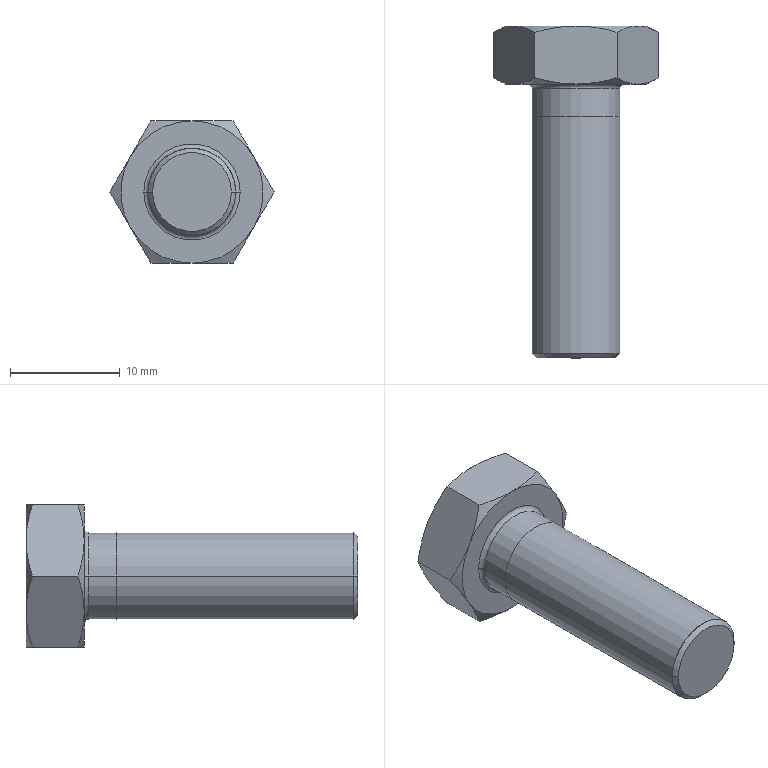Part | NX | features BREP 2 | 1 solid | 31 faces | box 15.011 x 30.3 x 13 mm | volume 2414 mm3 | cone 14 | plane 11 | cylinder 4 | torus 2 | commonest cylinder face diameters 6.647 x2 8 x2